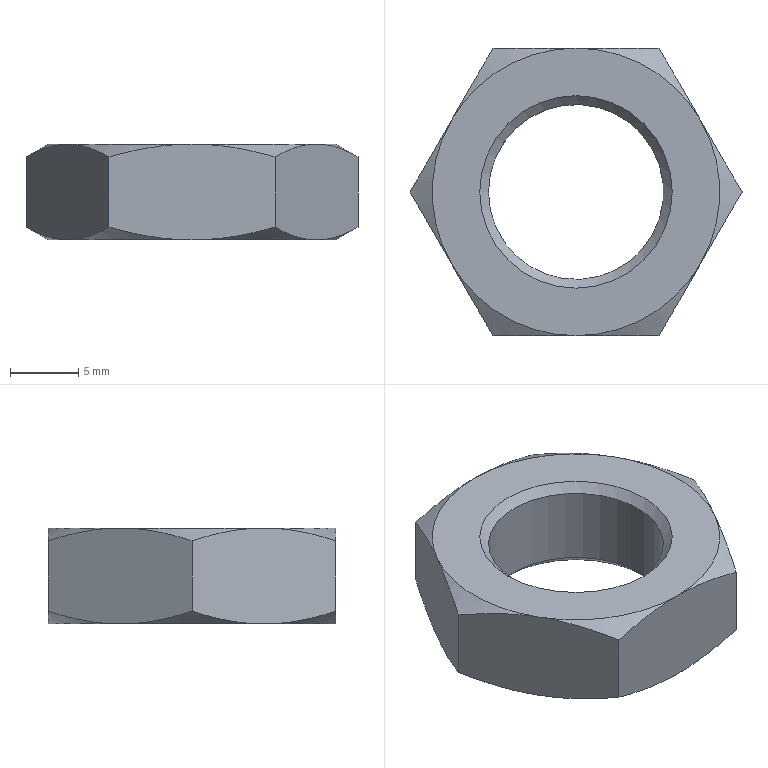Part | STEP file | Tube feed_id734_x_t | 1 solid | 23 faces | box 24.249 x 21 x 7 mm | volume 1738 mm3 | cone 14 | plane 8 | cylinder 1 | commonest cylinder face diameters 12.782 x1